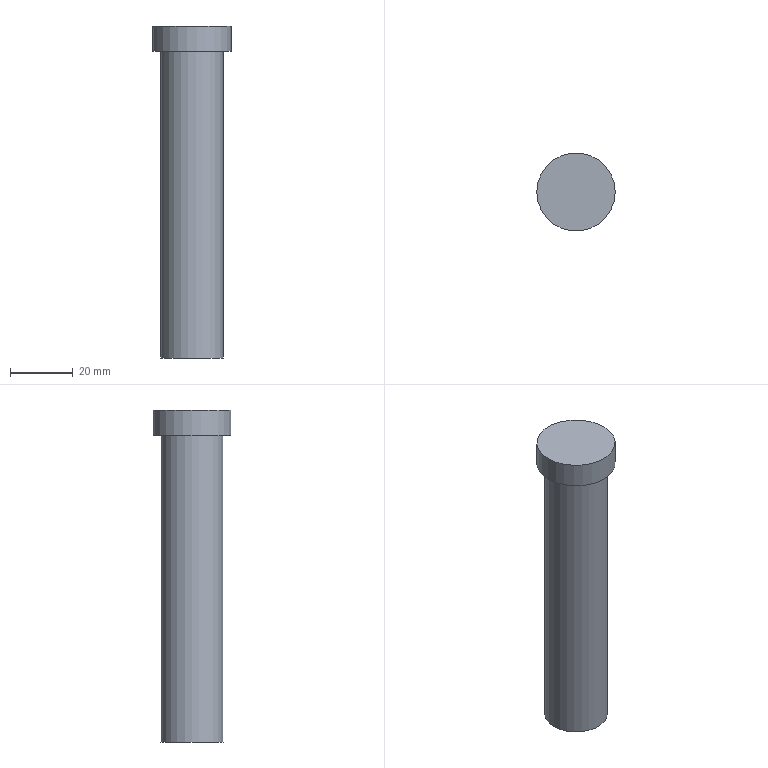Part | STEP file | solid 35 | 1 solid | 8 faces | box 25 x 25 x 106 mm | volume 34281 mm3 | plane 4 | cylinder 3 | cone 1 | commonest cylinder face diameters 6 x1 20 x1 25 x1